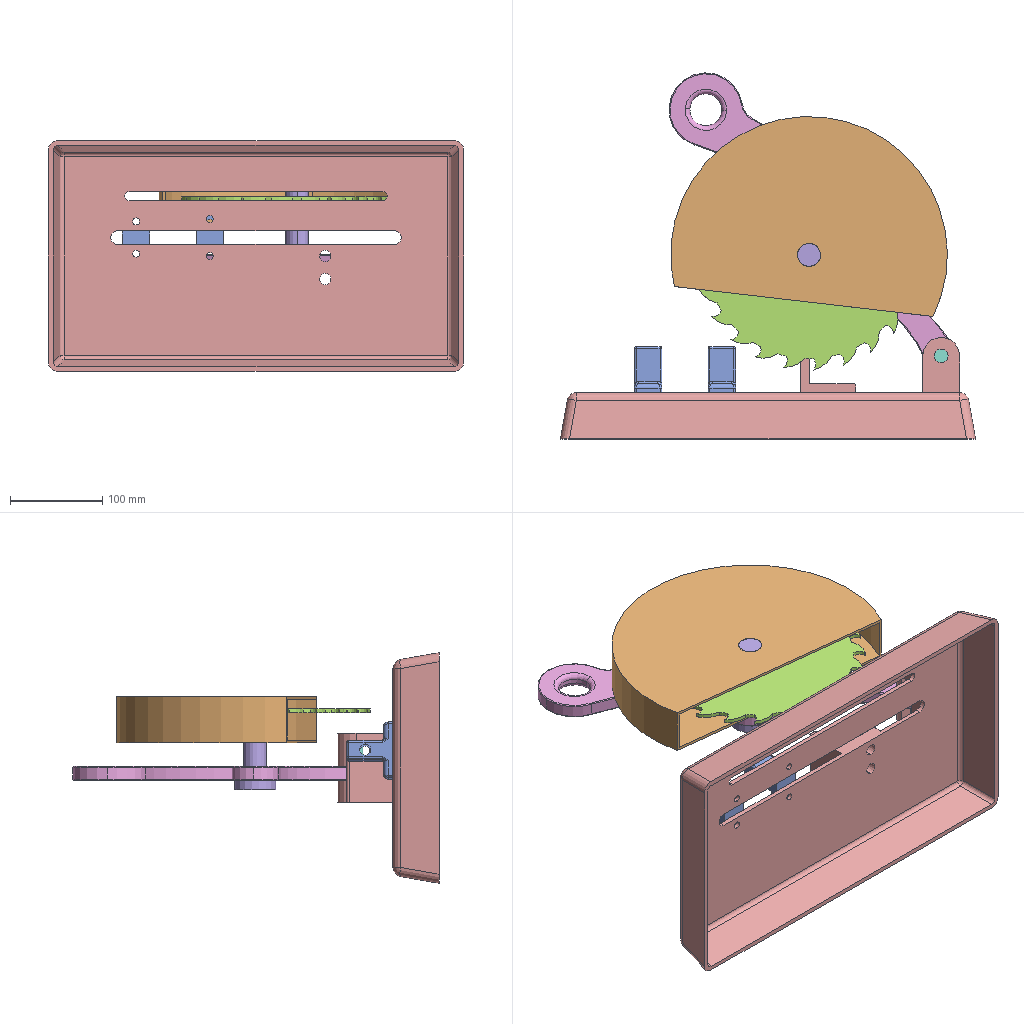Assembly | SolidWorks | 7 different items | 8 placed | box 450 x 397 x 250 mm
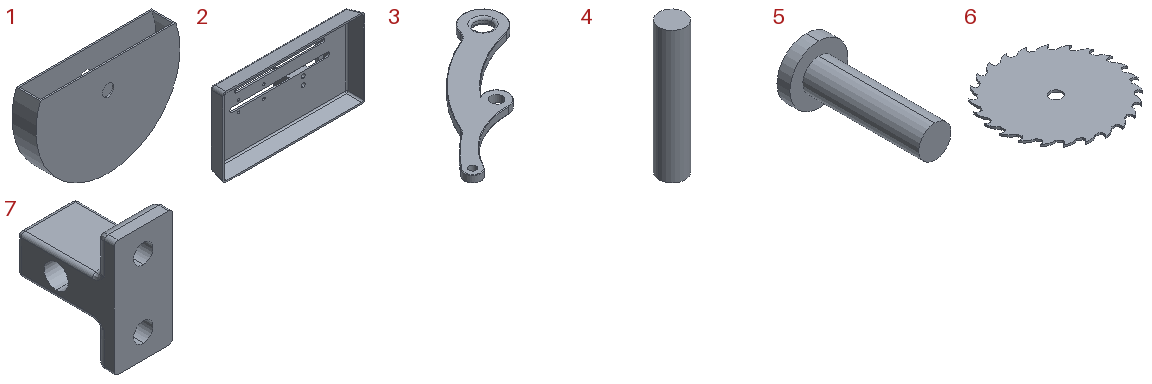Parts list (item | quantity | size | volume | features):
1 | x1 | 300 x 50 x 200.814 mm | 374070 mm3 | features Extrusion 1, ICE 1, Shell 1
2 | x1 | 450 x 110 x 250 mm | 893296 mm3 | features ICE 8, HoleWzd 4, Fillet 3, Extrusion 1
3 | x1 | 329.193 x 307.5 x 15 mm | 313638 mm3 | features Fillet 3, HoleWzd 3, Extrusion 1
4 | x1 | 15 x 15 x 75 mm | 13254 mm3 | features Revolution 1
5 | x1 | 45 x 100 x 45 mm | 60083 mm3 | features Extrusion 1, ICE 1
6 | x1 | 249.174 x 249.174 x 4 mm | 170975 mm3 | features Extrusion 1
7 | x2 | 30 x 50 x 60 mm | 35816 mm3 | features HoleWzd 3, Fillet 2, ICE 2, Chamfer 1, Extrusion 1
Mates (type | each side: item.copy, entity, surface, feature):
Concentric | 2.1 face cylinder Ø15.0 (15) Diameter Hole2 | 3.1 face cylinder Ø15.0 (15) Diameter Hole1
Concentric | 2.1 face cylinder Ø15.0 (15) Diameter Hole2 | 4.1 face cylinder Revolve1
Coincident | 2.1 face plane Boss-Extrude2 | 4.1 face plane Revolve1
Concentric | 6.1 face cylinder Boss-Extrude1 | 3.1 face cylinder Ø25.0 (25) Diameter Hole1
Concentric | 2.1 face cylinder Ø7.5 (7.5) Diameter Hole1 | 7.1 face cylinder Ø10.0 (10) Diameter Hole1 | 2 times
Coincident | 2.1 face plane Boss-Extrude1 | 7.1 face plane Boss-Extrude1
Concentric | 6.1 face cylinder Boss-Extrude1 | 1.1 face cylinder Cut-Extrude1
DistanceDim | 1.1 face plane Boss-Extrude1 | 3.1 face plane Boss-Extrude1
Coincident | 2.1 face plane Cut-Extrude6 | 6.1 face plane Boss-Extrude1
Concentric | 2.1 face cylinder Ø7.5 (7.5) Diameter Hole1 | 7.2 face cylinder Ø10.0 (10) Diameter Hole1
Parallel | 2.1 face cylinder Ø7.5 (7.5) Diameter Hole1 | 7.2 face cylinder Ø10.0 (10) Diameter Hole1
Coincident | 2.1 face plane Boss-Extrude1 | 7.2 face plane Boss-Extrude1
Concentric | 3.1 face cylinder Ø25.0 (25) Diameter Hole1 | 5.1 face cylinder Boss-Extrude1
Coincident | 3.1 face plane Boss-Extrude1 | 5.1 face plane Boss-Extrude2
DistanceDim | 3.1 face plane Boss-Extrude1 | 2.1 face plane Boss-Extrude2